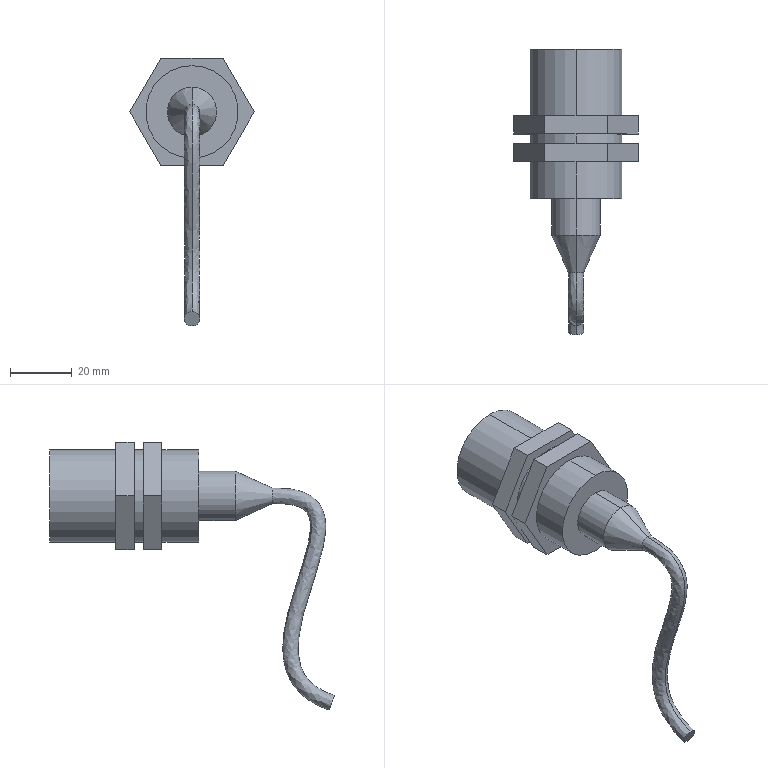Part | SolidWorks | features Boss 2, Extrusion 1, LPattern 1, Revolution 1, Sweep 1 | 1 solid | 31 faces | box 40.415 x 92.567 x 87.046 mm | volume 43733 mm3 | plane 19 | cylinder 8 | spline 2 | cone 2 | commonest cylinder face diameters 30 x6 16 x2
STEP:
#1=CARTESIAN_POINT('',(0.,-24.,-2.5));
#2=VERTEX_POINT('',#1);
#3=CARTESIAN_POINT('',(0.,-24.,2.5));
#4=VERTEX_POINT('',#3);
#5=CARTESIAN_POINT('',(0.,-24.,0.));
#6=DIRECTION('',(0.,-1.,0.));
#7=DIRECTION('',(0.,0.,-1.));
#8=AXIS2_PLACEMENT_3D('',#5,#6,#7);
#9=CIRCLE('',#8,2.5);
#10=EDGE_CURVE('',#2,#4,#9,.T.);
#11=ORIENTED_EDGE('',*,*,#10,.T.);
#12=CARTESIAN_POINT('',(0.,-44.067,-64.875));
#13=VERTEX_POINT('',#12);
#14=CARTESIAN_POINT('',(0.,-24.,2.5));
#15=CARTESIAN_POINT('',(0.,-26.65,2.597));
#16=CARTESIAN_POINT('',(0.,-28.95,2.46));
#17=CARTESIAN_POINT('',(0.,-32.981,1.702));
#18=CARTESIAN_POINT('',(0.,-34.722,1.075));
#19=CARTESIAN_POINT('',(0.,-37.648,-0.7421));
#20=CARTESIAN_POINT('',(0.,-38.817,-1.945));
#21=CARTESIAN_POINT('',(0.,-40.436,-4.701));
#22=CARTESIAN_POINT('',(0.,-40.89,-6.227));
#23=CARTESIAN_POINT('',(0.,-41.503,-10.943));
#24=CARTESIAN_POINT('',(0.,-40.983,-14.307));
#25=CARTESIAN_POINT('',(0.,-39.247,-21.447));
#26=CARTESIAN_POINT('',(0.,-37.999,-25.225));
#27=CARTESIAN_POINT('',(0.,-35.516,-32.906));
#28=CARTESIAN_POINT('',(0.,-34.279,-36.805));
#29=CARTESIAN_POINT('',(0.,-32.562,-44.284));
#30=CARTESIAN_POINT('',(0.,-32.091,-47.859));
#31=CARTESIAN_POINT('',(0.,-32.408,-52.584));
#32=CARTESIAN_POINT('',(0.,-32.68,-54.051));
#33=CARTESIAN_POINT('',(0.,-33.603,-56.751));
#34=CARTESIAN_POINT('',(0.,-34.251,-57.986));
#35=CARTESIAN_POINT('',(0.,-36.023,-60.274));
#36=CARTESIAN_POINT('',(0.,-37.151,-61.332));
#37=CARTESIAN_POINT('',(0.,-40.071,-63.265));
#38=CARTESIAN_POINT('',(0.,-41.867,-64.138));
#39=CARTESIAN_POINT('',(0.,-44.067,-64.875));
#40=B_SPLINE_CURVE_WITH_KNOTS('',3,(#14,#15,#16,#17,#18,#19,#20,#21,#22,#23,#24,#25,#26,#27,#28,#29,#30,#31,#32,#33,#34,#35,#36,#37,#38,#39),.UNSPECIFIED.,.F.,.F.,(4,2,2,2,2,2,2,2,2,2,2,2,4),(0.,0.0625,0.125,0.1875,0.25,0.375,0.5,0.625,0.75,0.8125,0.875,0.9375,1.),.UNSPECIFIED.);
#41=EDGE_CURVE('',#4,#13,#40,.T.);
#42=ORIENTED_EDGE('',*,*,#41,.T.);
#43=CARTESIAN_POINT('',(0.,-42.283,-69.546));
#44=VERTEX_POINT('',#43);
#45=CARTESIAN_POINT('',(0.,-43.175,-67.21));
#46=DIRECTION('',(0.,-0.9342,-0.3567));
#47=DIRECTION('',(0.,0.3567,-0.9342));
#48=AXIS2_PLACEMENT_3D('',#45,#46,#47);
#49=CIRCLE('',#48,2.5);
#50=EDGE_CURVE('',#44,#13,#49,.T.);
#51=ORIENTED_EDGE('',*,*,#50,.F.);
#52=CARTESIAN_POINT('',(0.,-24.,-2.5));
#53=CARTESIAN_POINT('',(0.,-26.373,-2.403));
#54=CARTESIAN_POINT('',(0.,-28.321,-2.523));
#55=CARTESIAN_POINT('',(0.,-31.428,-3.074));
#56=CARTESIAN_POINT('',(0.,-32.577,-3.503));
#57=CARTESIAN_POINT('',(0.,-34.264,-4.497));
#58=CARTESIAN_POINT('',(0.,-34.818,-5.05));
#59=CARTESIAN_POINT('',(0.,-35.671,-6.411));
#60=CARTESIAN_POINT('',(0.,-35.966,-7.244));
#61=CARTESIAN_POINT('',(0.,-36.423,-10.365));
#62=CARTESIAN_POINT('',(0.,-36.089,-13.236));
#63=CARTESIAN_POINT('',(0.,-34.517,-19.799));
#64=CARTESIAN_POINT('',(0.,-33.31,-23.491));
#65=CARTESIAN_POINT('',(0.,-30.816,-31.199));
#66=CARTESIAN_POINT('',(0.,-29.529,-35.22));
#67=CARTESIAN_POINT('',(0.,-27.663,-43.245));
#68=CARTESIAN_POINT('',(0.,-27.075,-47.254));
#69=CARTESIAN_POINT('',(0.,-27.418,-53.066));
#70=CARTESIAN_POINT('',(0.,-27.74,-54.971));
#71=CARTESIAN_POINT('',(0.,-28.945,-58.636));
#72=CARTESIAN_POINT('',(0.,-29.832,-60.395));
#73=CARTESIAN_POINT('',(0.,-32.262,-63.619));
#74=CARTESIAN_POINT('',(0.,-33.802,-65.079));
#75=CARTESIAN_POINT('',(0.,-37.539,-67.606));
#76=CARTESIAN_POINT('',(0.,-39.735,-68.676));
#77=CARTESIAN_POINT('',(0.,-42.283,-69.546));
#78=B_SPLINE_CURVE_WITH_KNOTS('',3,(#52,#53,#54,#55,#56,#57,#58,#59,#60,#61,#62,#63,#64,#65,#66,#67,#68,#69,#70,#71,#72,#73,#74,#75,#76,#77),.UNSPECIFIED.,.F.,.F.,(4,2,2,2,2,2,2,2,2,2,2,2,4),(0.,0.0625,0.125,0.1875,0.25,0.375,0.5,0.625,0.75,0.8125,0.875,0.9375,1.),.UNSPECIFIED.);
#79=EDGE_CURVE('',#2,#44,#78,.T.);
#80=ORIENTED_EDGE('',*,*,#79,.F.);
#81=EDGE_LOOP('',(#11,#42,#51,#80));
#82=FACE_OUTER_BOUND('',#81,.T.);
#83=CARTESIAN_POINT('',(0.,-24.,-2.5));
#84=CARTESIAN_POINT('',(0.,-26.373,-2.403));
#85=CARTESIAN_POINT('',(0.,-28.321,-2.523));
#86=CARTESIAN_POINT('',(0.,-31.428,-3.074));
#87=CARTESIAN_POINT('',(0.,-32.577,-3.503));
#88=CARTESIAN_POINT('',(0.,-34.264,-4.497));
#89=CARTESIAN_POINT('',(0.,-34.818,-5.05));
#90=CARTESIAN_POINT('',(0.,-35.671,-6.411));
#91=CARTESIAN_POINT('',(0.,-35.966,-7.244));
#92=CARTESIAN_POINT('',(0.,-36.423,-10.365));
#93=CARTESIAN_POINT('',(0.,-36.089,-13.236));
#94=CARTESIAN_POINT('',(0.,-34.517,-19.799));
#95=CARTESIAN_POINT('',(0.,-33.31,-23.491));
#96=CARTESIAN_POINT('',(0.,-30.816,-31.199));
#97=CARTESIAN_POINT('',(0.,-29.529,-35.22));
#98=CARTESIAN_POINT('',(0.,-27.663,-43.245));
#99=CARTESIAN_POINT('',(0.,-27.075,-47.254));
#100=CARTESIAN_POINT('',(0.,-27.418,-53.066));
#101=CARTESIAN_POINT('',(0.,-27.74,-54.971));
#102=CARTESIAN_POINT('',(0.,-28.945,-58.636));
#103=CARTESIAN_POINT('',(0.,-29.832,-60.395));
#104=CARTESIAN_POINT('',(0.,-32.262,-63.619));
#105=CARTESIAN_POINT('',(0.,-33.802,-65.079));
#106=CARTESIAN_POINT('',(0.,-37.539,-67.606));
#107=CARTESIAN_POINT('',(0.,-39.735,-68.676));
#108=CARTESIAN_POINT('',(0.,-42.283,-69.546));
#109=CARTESIAN_POINT('',(5.,-24.,-2.5));
#110=CARTESIAN_POINT('',(5.,-26.373,-2.403));
#111=CARTESIAN_POINT('',(5.,-28.321,-2.523));
#112=CARTESIAN_POINT('',(5.,-31.428,-3.074));
#113=CARTESIAN_POINT('',(5.,-32.577,-3.503));
#114=CARTESIAN_POINT('',(5.,-34.264,-4.497));
#115=CARTESIAN_POINT('',(5.,-34.818,-5.05));
#116=CARTESIAN_POINT('',(5.,-35.671,-6.411));
#117=CARTESIAN_POINT('',(5.,-35.966,-7.244));
#118=CARTESIAN_POINT('',(5.,-36.423,-10.365));
#119=CARTESIAN_POINT('',(5.,-36.089,-13.236));
#120=CARTESIAN_POINT('',(5.,-34.517,-19.799));
#121=CARTESIAN_POINT('',(5.,-33.31,-23.491));
#122=CARTESIAN_POINT('',(5.,-30.816,-31.199));
#123=CARTESIAN_POINT('',(5.,-29.529,-35.22));
#124=CARTESIAN_POINT('',(5.,-27.663,-43.245));
#125=CARTESIAN_POINT('',(5.,-27.075,-47.254));
#126=CARTESIAN_POINT('',(5.,-27.418,-53.066));
#127=CARTESIAN_POINT('',(5.,-27.74,-54.971));
#128=CARTESIAN_POINT('',(5.,-28.945,-58.636));
#129=CARTESIAN_POINT('',(5.,-29.832,-60.395));
#130=CARTESIAN_POINT('',(5.,-32.262,-63.619));
#131=CARTESIAN_POINT('',(5.,-33.802,-65.079));
#132=CARTESIAN_POINT('',(5.,-37.539,-67.606));
#133=CARTESIAN_POINT('',(5.,-39.735,-68.676));
#134=CARTESIAN_POINT('',(5.,-42.283,-69.546));
#135=CARTESIAN_POINT('',(5.,-24.,2.5));
#136=CARTESIAN_POINT('',(5.,-26.65,2.597));
#137=CARTESIAN_POINT('',(5.,-28.95,2.46));
#138=CARTESIAN_POINT('',(5.,-32.981,1.702));
#139=CARTESIAN_POINT('',(5.,-34.722,1.075));
#140=CARTESIAN_POINT('',(5.,-37.648,-0.7421));
#141=CARTESIAN_POINT('',(5.,-38.817,-1.945));
#142=CARTESIAN_POINT('',(5.,-40.436,-4.701));
#143=CARTESIAN_POINT('',(5.,-40.89,-6.227));
#144=CARTESIAN_POINT('',(5.,-41.503,-10.943));
#145=CARTESIAN_POINT('',(5.,-40.983,-14.307));
#146=CARTESIAN_POINT('',(5.,-39.247,-21.447));
#147=CARTESIAN_POINT('',(5.,-37.999,-25.225));
#148=CARTESIAN_POINT('',(5.,-35.516,-32.906));
#149=CARTESIAN_POINT('',(5.,-34.279,-36.805));
#150=CARTESIAN_POINT('',(5.,-32.562,-44.284));
#151=CARTESIAN_POINT('',(5.,-32.091,-47.859));
#152=CARTESIAN_POINT('',(5.,-32.408,-52.584));
#153=CARTESIAN_POINT('',(5.,-32.68,-54.051));
#154=CARTESIAN_POINT('',(5.,-33.603,-56.751));
#155=CARTESIAN_POINT('',(5.,-34.251,-57.986));
#156=CARTESIAN_POINT('',(5.,-36.023,-60.274));
#157=CARTESIAN_POINT('',(5.,-37.151,-61.332));
#158=CARTESIAN_POINT('',(5.,-40.071,-63.265));
#159=CARTESIAN_POINT('',(5.,-41.867,-64.138));
#160=CARTESIAN_POINT('',(5.,-44.067,-64.875));
#161=CARTESIAN_POINT('',(0.,-24.,2.5));
#162=CARTESIAN_POINT('',(0.,-26.65,2.597));
#163=CARTESIAN_POINT('',(0.,-28.95,2.46));
#164=CARTESIAN_POINT('',(0.,-32.981,1.702));
#165=CARTESIAN_POINT('',(0.,-34.722,1.075));
#166=CARTESIAN_POINT('',(0.,-37.648,-0.7421));
#167=CARTESIAN_POINT('',(0.,-38.817,-1.945));
#168=CARTESIAN_POINT('',(0.,-40.436,-4.701));
#169=CARTESIAN_POINT('',(0.,-40.89,-6.227));
#170=CARTESIAN_POINT('',(0.,-41.503,-10.943));
#171=CARTESIAN_POINT('',(0.,-40.983,-14.307));
#172=CARTESIAN_POINT('',(0.,-39.247,-21.447));
#173=CARTESIAN_POINT('',(0.,-37.999,-25.225));
#174=CARTESIAN_POINT('',(0.,-35.516,-32.906));
#175=CARTESIAN_POINT('',(0.,-34.279,-36.805));
#176=CARTESIAN_POINT('',(0.,-32.562,-44.284));
#177=CARTESIAN_POINT('',(0.,-32.091,-47.859));
#178=CARTESIAN_POINT('',(0.,-32.408,-52.584));
#179=CARTESIAN_POINT('',(0.,-32.68,-54.051));
#180=CARTESIAN_POINT('',(0.,-33.603,-56.751));
#181=CARTESIAN_POINT('',(0.,-34.251,-57.986));
#182=CARTESIAN_POINT('',(0.,-36.023,-60.274));
#183=CARTESIAN_POINT('',(0.,-37.151,-61.332));
#184=CARTESIAN_POINT('',(0.,-40.071,-63.265));
#185=CARTESIAN_POINT('',(0.,-41.867,-64.138));
#186=CARTESIAN_POINT('',(0.,-44.067,-64.875));
#187=CARTESIAN_POINT('',(-5.,-24.,2.5));
#188=CARTESIAN_POINT('',(-5.,-26.65,2.597));
#189=CARTESIAN_POINT('',(-5.,-28.95,2.46));
#190=CARTESIAN_POINT('',(-5.,-32.981,1.702));
#191=CARTESIAN_POINT('',(-5.,-34.722,1.075));
#192=CARTESIAN_POINT('',(-5.,-37.648,-0.7421));
#193=CARTESIAN_POINT('',(-5.,-38.817,-1.945));
#194=CARTESIAN_POINT('',(-5.,-40.436,-4.701));
#195=CARTESIAN_POINT('',(-5.,-40.89,-6.227));
#196=CARTESIAN_POINT('',(-5.,-41.503,-10.943));
#197=CARTESIAN_POINT('',(-5.,-40.983,-14.307));
#198=CARTESIAN_POINT('',(-5.,-39.247,-21.447));
#199=CARTESIAN_POINT('',(-5.,-37.999,-25.225));
#200=CARTESIAN_POINT('',(-5.,-35.516,-32.906));
#201=CARTESIAN_POINT('',(-5.,-34.279,-36.805));
#202=CARTESIAN_POINT('',(-5.,-32.562,-44.284));
#203=CARTESIAN_POINT('',(-5.,-32.091,-47.859));
#204=CARTESIAN_POINT('',(-5.,-32.408,-52.584));
#205=CARTESIAN_POINT('',(-5.,-32.68,-54.051));
#206=CARTESIAN_POINT('',(-5.,-33.603,-56.751));
#207=CARTESIAN_POINT('',(-5.,-34.251,-57.986));
#208=CARTESIAN_POINT('',(-5.,-36.023,-60.274));
#209=CARTESIAN_POINT('',(-5.,-37.151,-61.332));
#210=CARTESIAN_POINT('',(-5.,-40.071,-63.265));
#211=CARTESIAN_POINT('',(-5.,-41.867,-64.138));
#212=CARTESIAN_POINT('',(-5.,-44.067,-64.875));
#213=CARTESIAN_POINT('',(-5.,-24.,-2.5));
#214=CARTESIAN_POINT('',(-5.,-26.373,-2.403));
#215=CARTESIAN_POINT('',(-5.,-28.321,-2.523));
#216=CARTESIAN_POINT('',(-5.,-31.428,-3.074));
#217=CARTESIAN_POINT('',(-5.,-32.577,-3.503));
#218=CARTESIAN_POINT('',(-5.,-34.264,-4.497));
#219=CARTESIAN_POINT('',(-5.,-34.818,-5.05));
#220=CARTESIAN_POINT('',(-5.,-35.671,-6.411));
#221=CARTESIAN_POINT('',(-5.,-35.966,-7.244));
#222=CARTESIAN_POINT('',(-5.,-36.423,-10.365));
#223=CARTESIAN_POINT('',(-5.,-36.089,-13.236));
#224=CARTESIAN_POINT('',(-5.,-34.517,-19.799));
#225=CARTESIAN_POINT('',(-5.,-33.31,-23.491));
#226=CARTESIAN_POINT('',(-5.,-30.816,-31.199));
#227=CARTESIAN_POINT('',(-5.,-29.529,-35.22));
#228=CARTESIAN_POINT('',(-5.,-27.663,-43.245));
#229=CARTESIAN_POINT('',(-5.,-27.075,-47.254));
#230=CARTESIAN_POINT('',(-5.,-27.418,-53.066));
#231=CARTESIAN_POINT('',(-5.,-27.74,-54.971));
#232=CARTESIAN_POINT('',(-5.,-28.945,-58.636));
#233=CARTESIAN_POINT('',(-5.,-29.832,-60.395));
#234=CARTESIAN_POINT('',(-5.,-32.262,-63.619));
#235=CARTESIAN_POINT('',(-5.,-33.802,-65.079));
#236=CARTESIAN_POINT('',(-5.,-37.539,-67.606));
#237=CARTESIAN_POINT('',(-5.,-39.735,-68.676));
#238=CARTESIAN_POINT('',(-5.,-42.283,-69.546));
#239=CARTESIAN_POINT('',(0.,-24.,-2.5));
#240=CARTESIAN_POINT('',(0.,-26.373,-2.403));
#241=CARTESIAN_POINT('',(0.,-28.321,-2.523));
#242=CARTESIAN_POINT('',(0.,-31.428,-3.074));
#243=CARTESIAN_POINT('',(0.,-32.577,-3.503));
#244=CARTESIAN_POINT('',(0.,-34.264,-4.497));
#245=CARTESIAN_POINT('',(0.,-34.818,-5.05));
#246=CARTESIAN_POINT('',(0.,-35.671,-6.411));
#247=CARTESIAN_POINT('',(0.,-35.966,-7.244));
#248=CARTESIAN_POINT('',(0.,-36.423,-10.365));
#249=CARTESIAN_POINT('',(0.,-36.089,-13.236));
#250=CARTESIAN_POINT('',(0.,-34.517,-19.799));
#251=CARTESIAN_POINT('',(0.,-33.31,-23.491));
#252=CARTESIAN_POINT('',(0.,-30.816,-31.199));
#253=CARTESIAN_POINT('',(0.,-29.529,-35.22));
#254=CARTESIAN_POINT('',(0.,-27.663,-43.245));
#255=CARTESIAN_POINT('',(0.,-27.075,-47.254));
#256=CARTESIAN_POINT('',(0.,-27.418,-53.066));
#257=CARTESIAN_POINT('',(0.,-27.74,-54.971));
#258=CARTESIAN_POINT('',(0.,-28.945,-58.636));
#259=CARTESIAN_POINT('',(0.,-29.832,-60.395));
#260=CARTESIAN_POINT('',(0.,-32.262,-63.619));
#261=CARTESIAN_POINT('',(0.,-33.802,-65.079));
#262=CARTESIAN_POINT('',(0.,-37.539,-67.606));
#263=CARTESIAN_POINT('',(0.,-39.735,-68.676));
#264=CARTESIAN_POINT('',(0.,-42.283,-69.546));
#265=(BOUNDED_SURFACE()B_SPLINE_SURFACE(3,3,((#83,#84,#85,#86,#87,#88,#89,#90,#91,#92,#93,#94,#95,#96,#97,#98,#99,#100,#101,#102,#103,#104,#105,#106,#107,#108),(#109,#110,#111,#112,#113,#114,#115,#116,#117,#118,#119,#120,#121,#122,#123,#124,#125,#126,#127,#128,#129,#130,#131,#132,#133,#134),(#135,#136,#137,#138,#139,#140,#141,#142,#143,#144,#145,#146,#147,#148,#149,#150,#151,#152,#153,#154,#155,#156,#157,#158,#159,#160),(#161,#162,#163,#164,#165,#166,#167,#168,#169,#170,#171,#172,#173,#174,#175,#176,#177,#178,#179,#180,#181,#182,#183,#184,#185,#186),(#187,#188,#189,#190,#191,#192,#193,#194,#195,#196,#197,#198,#199,#200,#201,#202,#203,#204,#205,#206,#207,#208,#209,#210,#211,#212),(#213,#214,#215,#216,#217,#218,#219,#220,#221,#222,#223,#224,#225,#226,#227,#228,#229,#230,#231,#232,#233,#234,#235,#236,#237,#238),(#239,#240,#241,#242,#243,#244,#245,#246,#247,#248,#249,#250,#251,#252,#253,#254,#255,#256,#257,#258,#259,#260,#261,#262,#263,#264)),.UNSPECIFIED.,.T.,.F.,.F.)B_SPLINE_SURFACE_WITH_KNOTS((4,3,4),(4,2,2,2,2,2,2,2,2,2,2,2,4),(0.,0.5,1.),(0.,0.0625,0.125,0.1875,0.25,0.375,0.5,0.625,0.75,0.8125,0.875,0.9375,1.),.UNSPECIFIED.)GEOMETRIC_REPRESENTATION_ITEM()RATIONAL_B_SPLINE_SURFACE(((1.,1.,1.,1.,1.,1.,1.,1.,1.,1.,1.,1.,1.,1.,1.,1.,1.,1.,1.,1.,1.,1.,1.,1.,1.,1.),(0.3333,0.3333,0.3333,0.3333,0.3333,0.3333,0.3333,0.3333,0.3333,0.3333,0.3333,0.3333,0.3333,0.3333,0.3333,0.3333,0.3333,0.3333,0.3333,0.3333,0.3333,0.3333,0.3333,0.3333,0.3333,0.3333),(0.3333,0.3333,0.3333,0.3333,0.3333,0.3333,0.3333,0.3333,0.3333,0.3333,0.3333,0.3333,0.3333,0.3333,0.3333,0.3333,0.3333,0.3333,0.3333,0.3333,0.3333,0.3333,0.3333,0.3333,0.3333,0.3333),(1.,1.,1.,1.,1.,1.,1.,1.,1.,1.,1.,1.,1.,1.,1.,1.,1.,1.,1.,1.,1.,1.,1.,1.,1.,1.),(0.3333,0.3333,0.3333,0.3333,0.3333,0.3333,0.3333,0.3333,0.3333,0.3333,0.3333,0.3333,0.3333,0.3333,0.3333,0.3333,0.3333,0.3333,0.3333,0.3333,0.3333,0.3333,0.3333,0.3333,0.3333,0.3333),(0.3333,0.3333,0.3333,0.3333,0.3333,0.3333,0.3333,0.3333,0.3333,0.3333,0.3333,0.3333,0.3333,0.3333,0.3333,0.3333,0.3333,0.3333,0.3333,0.3333,0.3333,0.3333,0.3333,0.3333,0.3333,0.3333),(1.,1.,1.,1.,1.,1.,1.,1.,1.,1.,1.,1.,1.,1.,1.,1.,1.,1.,1.,1.,1.,1.,1.,1.,1.,1.)))REPRESENTATION_ITEM('')SURFACE());
#266=ADVANCED_FACE('',(#82),#265,.T.);
#267=ORIENTED_EDGE('',*,*,#10,.F.);
#268=CARTESIAN_POINT('',(0.,-11.832,-8.));
#269=VERTEX_POINT('',#268);
#270=CARTESIAN_POINT('',(0.,-24.,-2.5));
#271=DIRECTION('',(0.,0.9112,-0.4119));
#272=VECTOR('',#271,1000.);
#273=LINE('',#270,#272);
#274=EDGE_CURVE('',#2,#269,#273,.T.);
#275=ORIENTED_EDGE('',*,*,#274,.T.);
#276=CARTESIAN_POINT('',(0.,-11.832,8.));
#277=VERTEX_POINT('',#276);
#278=CARTESIAN_POINT('',(0.,-11.832,0.));
#279=DIRECTION('',(0.,1.,0.));
#280=DIRECTION('',(0.,0.,1.));
#281=AXIS2_PLACEMENT_3D('',#278,#279,#280);
#282=CIRCLE('',#281,8.);
#283=EDGE_CURVE('',#277,#269,#282,.T.);
#284=ORIENTED_EDGE('',*,*,#283,.F.);
#285=CARTESIAN_POINT('',(0.,-24.,2.5));
#286=DIRECTION('',(0.,0.9112,0.4119));
#287=VECTOR('',#286,1000.);
#288=LINE('',#285,#287);
#289=EDGE_CURVE('',#4,#277,#288,.T.);
#290=ORIENTED_EDGE('',*,*,#289,.F.);
#291=EDGE_LOOP('',(#267,#275,#284,#290));
#292=FACE_OUTER_BOUND('',#291,.T.);
#293=CARTESIAN_POINT('',(0.,-24.,0.));
#294=DIRECTION('',(0.,1.,0.));
#295=DIRECTION('',(0.,0.,1.));
#296=AXIS2_PLACEMENT_3D('',#293,#294,#295);
#297=CONICAL_SURFACE('',#296,2.5,0.4245);
#298=ADVANCED_FACE('',(#292),#297,.T.);
#299=ORIENTED_EDGE('',*,*,#283,.T.);
#300=CARTESIAN_POINT('',(0.,0.,-8.));
#301=VERTEX_POINT('',#300);
#302=CARTESIAN_POINT('',(0.,0.,-8.));
#303=DIRECTION('',(0.,1.,0.));
#304=VECTOR('',#303,1000.);
#305=LINE('',#302,#304);
#306=EDGE_CURVE('',#269,#301,#305,.T.);
#307=ORIENTED_EDGE('',*,*,#306,.T.);
#308=CARTESIAN_POINT('',(0.,0.,8.));
#309=VERTEX_POINT('',#308);
#310=CARTESIAN_POINT('',(0.,0.,0.));
#311=DIRECTION('',(0.,-1.,0.));
#312=DIRECTION('',(0.,0.,1.));
#313=AXIS2_PLACEMENT_3D('',#310,#311,#312);
#314=CIRCLE('',#313,8.);
#315=EDGE_CURVE('',#301,#309,#314,.T.);
#316=ORIENTED_EDGE('',*,*,#315,.T.);
#317=CARTESIAN_POINT('',(0.,0.,8.));
#318=DIRECTION('',(0.,1.,0.));
#319=VECTOR('',#318,1000.);
#320=LINE('',#317,#319);
#321=EDGE_CURVE('',#277,#309,#320,.T.);
#322=ORIENTED_EDGE('',*,*,#321,.F.);
#323=EDGE_LOOP('',(#299,#307,#316,#322));
#324=FACE_OUTER_BOUND('',#323,.T.);
#325=CARTESIAN_POINT('',(0.,0.,0.));
#326=DIRECTION('',(0.,1.,0.));
#327=DIRECTION('',(0.,0.,1.));
#328=AXIS2_PLACEMENT_3D('',#325,#326,#327);
#329=CYLINDRICAL_SURFACE('',#328,8.);
#330=ADVANCED_FACE('',(#324),#329,.T.);
#331=CARTESIAN_POINT('',(0.,48.5,15.));
#332=VERTEX_POINT('',#331);
#333=CARTESIAN_POINT('',(0.,48.5,-15.));
#334=VERTEX_POINT('',#333);
#335=CARTESIAN_POINT('',(0.,48.5,0.));
#336=DIRECTION('',(0.,1.,0.));
#337=DIRECTION('',(0.,0.,1.));
#338=AXIS2_PLACEMENT_3D('',#335,#336,#337);
#339=CIRCLE('',#338,15.);
#340=EDGE_CURVE('',#332,#334,#339,.T.);
#341=ORIENTED_EDGE('',*,*,#340,.F.);
#342=CARTESIAN_POINT('',(0.,27.,15.));
#343=VERTEX_POINT('',#342);
#344=CARTESIAN_POINT('',(0.,48.5,15.));
#345=DIRECTION('',(0.,-1.,0.));
#346=VECTOR('',#345,1000.);
#347=LINE('',#344,#346);
#348=EDGE_CURVE('',#332,#343,#347,.T.);
#349=ORIENTED_EDGE('',*,*,#348,.T.);
#350=CARTESIAN_POINT('',(0.,27.,-15.));
#351=VERTEX_POINT('',#350);
#352=CARTESIAN_POINT('',(0.,27.,0.));
#353=DIRECTION('',(0.,1.,0.));
#354=DIRECTION('',(0.,0.,1.));
#355=AXIS2_PLACEMENT_3D('',#352,#353,#354);
#356=CIRCLE('',#355,15.);
#357=EDGE_CURVE('',#343,#351,#356,.T.);
#358=ORIENTED_EDGE('',*,*,#357,.T.);
#359=CARTESIAN_POINT('',(0.,48.5,-15.));
#360=DIRECTION('',(0.,-1.,0.));
#361=VECTOR('',#360,1000.);
#362=LINE('',#359,#361);
#363=EDGE_CURVE('',#334,#351,#362,.T.);
#364=ORIENTED_EDGE('',*,*,#363,.F.);
#365=EDGE_LOOP('',(#341,#349,#358,#364));
#366=FACE_OUTER_BOUND('',#365,.T.);
#367=CARTESIAN_POINT('',(0.,48.5,0.));
#368=DIRECTION('',(0.,-1.,0.));
#369=DIRECTION('',(0.,0.,-1.));
#370=AXIS2_PLACEMENT_3D('',#367,#368,#369);
#371=CYLINDRICAL_SURFACE('',#370,15.);
#372=ADVANCED_FACE('',(#366),#371,.T.);
#373=CARTESIAN_POINT('',(0.,12.,15.));
#374=VERTEX_POINT('',#373);
#375=CARTESIAN_POINT('',(0.,12.,-15.));
#376=VERTEX_POINT('',#375);
#377=CARTESIAN_POINT('',(0.,12.,0.));
#378=DIRECTION('',(0.,1.,0.));
#379=DIRECTION('',(0.,0.,1.));
#380=AXIS2_PLACEMENT_3D('',#377,#378,#379);
#381=CIRCLE('',#380,15.);
#382=EDGE_CURVE('',#374,#376,#381,.T.);
#383=ORIENTED_EDGE('',*,*,#382,.F.);
#384=CARTESIAN_POINT('',(0.,0.,15.));
#385=VERTEX_POINT('',#384);
#386=CARTESIAN_POINT('',(0.,48.5,15.));
#387=DIRECTION('',(0.,-1.,0.));
#388=VECTOR('',#387,1000.);
#389=LINE('',#386,#388);
#390=EDGE_CURVE('',#374,#385,#389,.T.);
#391=ORIENTED_EDGE('',*,*,#390,.T.);
#392=CARTESIAN_POINT('',(0.,0.,-15.));
#393=VERTEX_POINT('',#392);
#394=CARTESIAN_POINT('',(0.,0.,0.));
#395=DIRECTION('',(0.,1.,0.));
#396=DIRECTION('',(0.,0.,1.));
#397=AXIS2_PLACEMENT_3D('',#394,#395,#396);
#398=CIRCLE('',#397,15.);
#399=EDGE_CURVE('',#385,#393,#398,.T.);
#400=ORIENTED_EDGE('',*,*,#399,.T.);
#401=CARTESIAN_POINT('',(0.,48.5,-15.));
#402=DIRECTION('',(0.,-1.,0.));
#403=VECTOR('',#402,1000.);
#404=LINE('',#401,#403);
#405=EDGE_CURVE('',#376,#393,#404,.T.);
#406=ORIENTED_EDGE('',*,*,#405,.F.);
#407=EDGE_LOOP('',(#383,#391,#400,#406));
#408=FACE_OUTER_BOUND('',#407,.T.);
#409=CARTESIAN_POINT('',(0.,48.5,0.));
#410=DIRECTION('',(0.,-1.,0.));
#411=DIRECTION('',(0.,0.,-1.));
#412=AXIS2_PLACEMENT_3D('',#409,#410,#411);
#413=CYLINDRICAL_SURFACE('',#412,15.);
#414=ADVANCED_FACE('',(#408),#413,.T.);
#415=CARTESIAN_POINT('',(0.,21.,15.));
#416=VERTEX_POINT('',#415);
#417=CARTESIAN_POINT('',(0.,21.,-15.));
#418=VERTEX_POINT('',#417);
#419=CARTESIAN_POINT('',(0.,21.,0.));
#420=DIRECTION('',(0.,1.,0.));
#421=DIRECTION('',(0.,0.,1.));
#422=AXIS2_PLACEMENT_3D('',#419,#420,#421);
#423=CIRCLE('',#422,15.);
#424=EDGE_CURVE('',#416,#418,#423,.T.);
#425=ORIENTED_EDGE('',*,*,#424,.F.);
#426=CARTESIAN_POINT('',(0.,18.,15.));
#427=VERTEX_POINT('',#426);
#428=CARTESIAN_POINT('',(0.,48.5,15.));
#429=DIRECTION('',(0.,-1.,0.));
#430=VECTOR('',#429,1000.);
#431=LINE('',#428,#430);
#432=EDGE_CURVE('',#416,#427,#431,.T.);
#433=ORIENTED_EDGE('',*,*,#432,.T.);
#434=CARTESIAN_POINT('',(0.,18.,-15.));
#435=VERTEX_POINT('',#434);
#436=CARTESIAN_POINT('',(0.,18.,0.));
#437=DIRECTION('',(0.,1.,0.));
#438=DIRECTION('',(0.,0.,1.));
#439=AXIS2_PLACEMENT_3D('',#436,#437,#438);
#440=CIRCLE('',#439,15.);
#441=EDGE_CURVE('',#427,#435,#440,.T.);
#442=ORIENTED_EDGE('',*,*,#441,.T.);
#443=CARTESIAN_POINT('',(0.,48.5,-15.));
#444=DIRECTION('',(0.,-1.,0.));
#445=VECTOR('',#444,1000.);
#446=LINE('',#443,#445);
#447=EDGE_CURVE('',#418,#435,#446,.T.);
#448=ORIENTED_EDGE('',*,*,#447,.F.);
#449=EDGE_LOOP('',(#425,#433,#442,#448));
#450=FACE_OUTER_BOUND('',#449,.T.);
#451=CARTESIAN_POINT('',(0.,48.5,0.));
#452=DIRECTION('',(0.,-1.,0.));
#453=DIRECTION('',(0.,0.,-1.));
#454=AXIS2_PLACEMENT_3D('',#451,#452,#453);
#455=CYLINDRICAL_SURFACE('',#454,15.);
#456=ADVANCED_FACE('',(#450),#455,.T.);
#457=CARTESIAN_POINT('',(0.,0.,0.));
#458=DIRECTION('',(0.,1.,0.));
#459=DIRECTION('',(0.,0.,1.));
#460=AXIS2_PLACEMENT_3D('',#457,#458,#459);
#461=CIRCLE('',#460,15.);
#462=EDGE_CURVE('',#393,#385,#461,.T.);
#463=ORIENTED_EDGE('',*,*,#462,.F.);
#464=ORIENTED_EDGE('',*,*,#399,.F.);
#465=EDGE_LOOP('',(#463,#464));
#466=FACE_OUTER_BOUND('',#465,.T.);
#467=CARTESIAN_POINT('',(0.,0.,0.));
#468=DIRECTION('',(0.,-1.,0.));
#469=DIRECTION('',(0.,0.,1.));
#470=AXIS2_PLACEMENT_3D('',#467,#468,#469);
#471=CIRCLE('',#470,8.);
#472=EDGE_CURVE('',#309,#301,#471,.T.);
#473=ORIENTED_EDGE('',*,*,#472,.F.);
#474=ORIENTED_EDGE('',*,*,#315,.F.);
#475=EDGE_LOOP('',(#473,#474));
#476=FACE_BOUND('',#475,.T.);
#477=CARTESIAN_POINT('',(0.,0.,0.));
#478=DIRECTION('',(0.,1.,0.));
#479=DIRECTION('',(0.,0.,1.));
#480=AXIS2_PLACEMENT_3D('',#477,#478,#479);
#481=PLANE('',#480);
#482=ADVANCED_FACE('',(#466,#476),#481,.F.);
#483=ORIENTED_EDGE('',*,*,#432,.F.);
#484=CARTESIAN_POINT('',(0.,21.,0.));
#485=DIRECTION('',(0.,1.,0.));
#486=DIRECTION('',(0.,0.,1.));
#487=AXIS2_PLACEMENT_3D('',#484,#485,#486);
#488=CIRCLE('',#487,15.);
#489=EDGE_CURVE('',#418,#416,#488,.T.);
#490=ORIENTED_EDGE('',*,*,#489,.F.);
#491=ORIENTED_EDGE('',*,*,#447,.T.);
#492=CARTESIAN_POINT('',(0.,18.,0.));
#493=DIRECTION('',(0.,1.,0.));
#494=DIRECTION('',(0.,0.,1.));
#495=AXIS2_PLACEMENT_3D('',#492,#493,#494);
#496=CIRCLE('',#495,15.);
#497=EDGE_CURVE('',#435,#427,#496,.T.);
#498=ORIENTED_EDGE('',*,*,#497,.T.);
#499=EDGE_LOOP('',(#483,#490,#491,#498));
#500=FACE_OUTER_BOUND('',#499,.T.);
#501=CARTESIAN_POINT('',(0.,48.5,0.));
#502=DIRECTION('',(0.,-1.,0.));
#503=DIRECTION('',(0.,0.,-1.));
#504=AXIS2_PLACEMENT_3D('',#501,#502,#503);
#505=CYLINDRICAL_SURFACE('',#504,15.);
#506=ADVANCED_FACE('',(#500),#505,.T.);
#507=CARTESIAN_POINT('',(-10.104,18.,17.5));
#508=VERTEX_POINT('',#507);
#509=CARTESIAN_POINT('',(10.104,18.,17.5));
#510=VERTEX_POINT('',#509);
#511=CARTESIAN_POINT('',(-10.104,18.,17.5));
#512=DIRECTION('',(1.,0.,0.));
#513=VECTOR('',#512,1000.);
#514=LINE('',#511,#513);
#515=EDGE_CURVE('',#508,#510,#514,.T.);
#516=ORIENTED_EDGE('',*,*,#515,.T.);
#517=CARTESIAN_POINT('',(20.207,18.,0.));
#518=VERTEX_POINT('',#517);
#519=CARTESIAN_POINT('',(10.104,18.,17.5));
#520=DIRECTION('',(0.5,0.,-0.866));
#521=VECTOR('',#520,1000.);
#522=LINE('',#519,#521);
#523=EDGE_CURVE('',#510,#518,#522,.T.);
#524=ORIENTED_EDGE('',*,*,#523,.T.);
#525=CARTESIAN_POINT('',(10.104,18.,-17.5));
#526=VERTEX_POINT('',#525);
#527=CARTESIAN_POINT('',(20.207,18.,0.));
#528=DIRECTION('',(-0.5,0.,-0.866));
#529=VECTOR('',#528,1000.);
#530=LINE('',#527,#529);
#531=EDGE_CURVE('',#518,#526,#530,.T.);
#532=ORIENTED_EDGE('',*,*,#531,.T.);
#533=CARTESIAN_POINT('',(-10.104,18.,-17.5));
#534=VERTEX_POINT('',#533);
#535=CARTESIAN_POINT('',(10.104,18.,-17.5));
#536=DIRECTION('',(-1.,0.,0.));
#537=VECTOR('',#536,1000.);
#538=LINE('',#535,#537);
#539=EDGE_CURVE('',#526,#534,#538,.T.);
#540=ORIENTED_EDGE('',*,*,#539,.T.);
#541=CARTESIAN_POINT('',(-20.207,18.,0.));
#542=VERTEX_POINT('',#541);
#543=CARTESIAN_POINT('',(-10.104,18.,-17.5));
#544=DIRECTION('',(-0.5,0.,0.866));
#545=VECTOR('',#544,1000.);
#546=LINE('',#543,#545);
#547=EDGE_CURVE('',#534,#542,#546,.T.);
#548=ORIENTED_EDGE('',*,*,#547,.T.);
#549=CARTESIAN_POINT('',(-20.207,18.,0.));
#550=DIRECTION('',(0.5,0.,0.866));
#551=VECTOR('',#550,1000.);
#552=LINE('',#549,#551);
#553=EDGE_CURVE('',#542,#508,#552,.T.);
#554=ORIENTED_EDGE('',*,*,#553,.T.);
#555=EDGE_LOOP('',(#516,#524,#532,#540,#548,#554));
#556=FACE_OUTER_BOUND('',#555,.T.);
#557=ORIENTED_EDGE('',*,*,#497,.F.);
#558=ORIENTED_EDGE('',*,*,#441,.F.);
#559=EDGE_LOOP('',(#557,#558));
#560=FACE_BOUND('',#559,.T.);
#561=CARTESIAN_POINT('',(10.104,18.,17.5));
#562=DIRECTION('',(0.,1.,0.));
#563=DIRECTION('',(0.,0.,1.));
#564=AXIS2_PLACEMENT_3D('',#561,#562,#563);
#565=PLANE('',#564);
#566=ADVANCED_FACE('',(#556,#560),#565,.T.);
#567=CARTESIAN_POINT('',(-10.104,12.,17.5));
#568=VERTEX_POINT('',#567);
#569=CARTESIAN_POINT('',(10.104,12.,17.5));
#570=VERTEX_POINT('',#569);
#571=CARTESIAN_POINT('',(-10.104,12.,17.5));
#572=DIRECTION('',(1.,0.,0.));
#573=VECTOR('',#572,1000.);
#574=LINE('',#571,#573);
#575=EDGE_CURVE('',#568,#570,#574,.T.);
#576=ORIENTED_EDGE('',*,*,#575,.F.);
#577=CARTESIAN_POINT('',(-20.207,12.,0.));
#578=VERTEX_POINT('',#577);
#579=CARTESIAN_POINT('',(-20.207,12.,0.));
#580=DIRECTION('',(0.5,0.,0.866));
#581=VECTOR('',#580,1000.);
#582=LINE('',#579,#581);
#583=EDGE_CURVE('',#578,#568,#582,.T.);
#584=ORIENTED_EDGE('',*,*,#583,.F.);
#585=CARTESIAN_POINT('',(-10.104,12.,-17.5));
#586=VERTEX_POINT('',#585);
#587=CARTESIAN_POINT('',(-10.104,12.,-17.5));
#588=DIRECTION('',(-0.5,0.,0.866));
#589=VECTOR('',#588,1000.);
#590=LINE('',#587,#589);
#591=EDGE_CURVE('',#586,#578,#590,.T.);
#592=ORIENTED_EDGE('',*,*,#591,.F.);
#593=CARTESIAN_POINT('',(10.104,12.,-17.5));
#594=VERTEX_POINT('',#593);
#595=CARTESIAN_POINT('',(10.104,12.,-17.5));
#596=DIRECTION('',(-1.,0.,0.));
#597=VECTOR('',#596,1000.);
#598=LINE('',#595,#597);
#599=EDGE_CURVE('',#594,#586,#598,.T.);
#600=ORIENTED_EDGE('',*,*,#599,.F.);
#601=CARTESIAN_POINT('',(20.207,12.,0.));
#602=VERTEX_POINT('',#601);
#603=CARTESIAN_POINT('',(20.207,12.,0.));
#604=DIRECTION('',(-0.5,0.,-0.866));
#605=VECTOR('',#604,1000.);
#606=LINE('',#603,#605);
#607=EDGE_CURVE('',#602,#594,#606,.T.);
#608=ORIENTED_EDGE('',*,*,#607,.F.);
#609=CARTESIAN_POINT('',(10.104,12.,17.5));
#610=DIRECTION('',(0.5,0.,-0.866));
#611=VECTOR('',#610,1000.);
#612=LINE('',#609,#611);
#613=EDGE_CURVE('',#570,#602,#612,.T.);
#614=ORIENTED_EDGE('',*,*,#613,.F.);
#615=EDGE_LOOP('',(#576,#584,#592,#600,#608,#614));
#616=FACE_OUTER_BOUND('',#615,.T.);
#617=CARTESIAN_POINT('',(0.,12.,0.));
#618=DIRECTION('',(0.,1.,0.));
#619=DIRECTION('',(0.,0.,1.));
#620=AXIS2_PLACEMENT_3D('',#617,#618,#619);
#621=CIRCLE('',#620,15.);
#622=EDGE_CURVE('',#376,#374,#621,.T.);
#623=ORIENTED_EDGE('',*,*,#622,.T.);
#624=ORIENTED_EDGE('',*,*,#382,.T.);
#625=EDGE_LOOP('',(#623,#624));
#626=FACE_BOUND('',#625,.T.);
#627=CARTESIAN_POINT('',(10.104,12.,17.5));
#628=DIRECTION('',(0.,1.,0.));
#629=DIRECTION('',(0.,0.,1.));
#630=AXIS2_PLACEMENT_3D('',#627,#628,#629);
#631=PLANE('',#630);
#632=ADVANCED_FACE('',(#616,#626),#631,.F.);
#633=ORIENTED_EDGE('',*,*,#575,.T.);
#634=CARTESIAN_POINT('',(10.104,18.,17.5));
#635=DIRECTION('',(0.,-1.,0.));
#636=VECTOR('',#635,1000.);
#637=LINE('',#634,#636);
#638=EDGE_CURVE('',#510,#570,#637,.T.);
#639=ORIENTED_EDGE('',*,*,#638,.F.);
#640=ORIENTED_EDGE('',*,*,#515,.F.);
#641=CARTESIAN_POINT('',(-10.104,18.,17.5));
#642=DIRECTION('',(0.,-1.,0.));
#643=VECTOR('',#642,1000.);
#644=LINE('',#641,#643);
#645=EDGE_CURVE('',#508,#568,#644,.T.);
#646=ORIENTED_EDGE('',*,*,#645,.T.);
#647=EDGE_LOOP('',(#633,#639,#640,#646));
#648=FACE_OUTER_BOUND('',#647,.T.);
#649=CARTESIAN_POINT('',(-10.104,18.,17.5));
#650=DIRECTION('',(0.,0.,-1.));
#651=DIRECTION('',(-1.,0.,0.));
#652=AXIS2_PLACEMENT_3D('',#649,#650,#651);
#653=PLANE('',#652);
#654=ADVANCED_FACE('',(#648),#653,.F.);
#655=ORIENTED_EDGE('',*,*,#613,.T.);
#656=CARTESIAN_POINT('',(20.207,18.,0.));
#657=DIRECTION('',(0.,-1.,0.));
#658=VECTOR('',#657,1000.);
#659=LINE('',#656,#658);
#660=EDGE_CURVE('',#518,#602,#659,.T.);
#661=ORIENTED_EDGE('',*,*,#660,.F.);
#662=ORIENTED_EDGE('',*,*,#523,.F.);
#663=ORIENTED_EDGE('',*,*,#638,.T.);
#664=EDGE_LOOP('',(#655,#661,#662,#663));
#665=FACE_OUTER_BOUND('',#664,.T.);
#666=CARTESIAN_POINT('',(10.104,18.,17.5));
#667=DIRECTION('',(-0.866,0.,-0.5));
#668=DIRECTION('',(-0.5,0.,0.866));
#669=AXIS2_PLACEMENT_3D('',#666,#667,#668);
#670=PLANE('',#669);
#671=ADVANCED_FACE('',(#665),#670,.F.);
#672=ORIENTED_EDGE('',*,*,#607,.T.);
#673=CARTESIAN_POINT('',(10.104,18.,-17.5));
#674=DIRECTION('',(0.,-1.,0.));
#675=VECTOR('',#674,1000.);
#676=LINE('',#673,#675);
#677=EDGE_CURVE('',#526,#594,#676,.T.);
#678=ORIENTED_EDGE('',*,*,#677,.F.);
#679=ORIENTED_EDGE('',*,*,#531,.F.);
#680=ORIENTED_EDGE('',*,*,#660,.T.);
#681=EDGE_LOOP('',(#672,#678,#679,#680));
#682=FACE_OUTER_BOUND('',#681,.T.);
#683=CARTESIAN_POINT('',(20.207,18.,0.));
#684=DIRECTION('',(-0.866,0.,0.5));
#685=DIRECTION('',(0.5,0.,0.866));
#686=AXIS2_PLACEMENT_3D('',#683,#684,#685);
#687=PLANE('',#686);
#688=ADVANCED_FACE('',(#682),#687,.F.);
#689=ORIENTED_EDGE('',*,*,#599,.T.);
#690=CARTESIAN_POINT('',(-10.104,18.,-17.5));
#691=DIRECTION('',(0.,-1.,0.));
#692=VECTOR('',#691,1000.);
#693=LINE('',#690,#692);
#694=EDGE_CURVE('',#534,#586,#693,.T.);
#695=ORIENTED_EDGE('',*,*,#694,.F.);
#696=ORIENTED_EDGE('',*,*,#539,.F.);
#697=ORIENTED_EDGE('',*,*,#677,.T.);
#698=EDGE_LOOP('',(#689,#695,#696,#697));
#699=FACE_OUTER_BOUND('',#698,.T.);
#700=CARTESIAN_POINT('',(10.104,18.,-17.5));
#701=DIRECTION('',(0.,0.,1.));
#702=DIRECTION('',(1.,0.,0.));
#703=AXIS2_PLACEMENT_3D('',#700,#701,#702);
#704=PLANE('',#703);
#705=ADVANCED_FACE('',(#699),#704,.F.);
#706=ORIENTED_EDGE('',*,*,#591,.T.);
#707=CARTESIAN_POINT('',(-20.207,18.,0.));
#708=DIRECTION('',(0.,-1.,0.));
#709=VECTOR('',#708,1000.);
#710=LINE('',#707,#709);
#711=EDGE_CURVE('',#542,#578,#710,.T.);
#712=ORIENTED_EDGE('',*,*,#711,.F.);
#713=ORIENTED_EDGE('',*,*,#547,.F.);
#714=ORIENTED_EDGE('',*,*,#694,.T.);
#715=EDGE_LOOP('',(#706,#712,#713,#714));
#716=FACE_OUTER_BOUND('',#715,.T.);
#717=CARTESIAN_POINT('',(-10.104,18.,-17.5));
#718=DIRECTION('',(0.866,0.,0.5));
#719=DIRECTION('',(0.5,0.,-0.866));
#720=AXIS2_PLACEMENT_3D('',#717,#718,#719);
#721=PLANE('',#720);
#722=ADVANCED_FACE('',(#716),#721,.F.);
#723=ORIENTED_EDGE('',*,*,#583,.T.);
#724=ORIENTED_EDGE('',*,*,#645,.F.);
#725=ORIENTED_EDGE('',*,*,#553,.F.);
#726=ORIENTED_EDGE('',*,*,#711,.T.);
#727=EDGE_LOOP('',(#723,#724,#725,#726));
#728=FACE_OUTER_BOUND('',#727,.T.);
#729=CARTESIAN_POINT('',(-20.207,18.,0.));
#730=DIRECTION('',(0.866,0.,-0.5));
#731=DIRECTION('',(-0.5,0.,-0.866));
#732=AXIS2_PLACEMENT_3D('',#729,#730,#731);
#733=PLANE('',#732);
#734=ADVANCED_FACE('',(#728),#733,.F.);
#735=ORIENTED_EDGE('',*,*,#390,.F.);
#736=ORIENTED_EDGE('',*,*,#622,.F.);
#737=ORIENTED_EDGE('',*,*,#405,.T.);
#738=ORIENTED_EDGE('',*,*,#462,.T.);
#739=EDGE_LOOP('',(#735,#736,#737,#738));
#740=FACE_OUTER_BOUND('',#739,.T.);
#741=CARTESIAN_POINT('',(0.,48.5,0.));
#742=DIRECTION('',(0.,-1.,0.));
#743=DIRECTION('',(0.,0.,-1.));
#744=AXIS2_PLACEMENT_3D('',#741,#742,#743);
#745=CYLINDRICAL_SURFACE('',#744,15.);
#746=ADVANCED_FACE('',(#740),#745,.T.);
#747=CARTESIAN_POINT('',(-10.104,27.,17.5));
#748=VERTEX_POINT('',#747);
#749=CARTESIAN_POINT('',(10.104,27.,17.5));
#750=VERTEX_POINT('',#749);
#751=CARTESIAN_POINT('',(-10.104,27.,17.5));
#752=DIRECTION('',(1.,0.,0.));
#753=VECTOR('',#752,1000.);
#754=LINE('',#751,#753);
#755=EDGE_CURVE('',#748,#750,#754,.T.);
#756=ORIENTED_EDGE('',*,*,#755,.T.);
#757=CARTESIAN_POINT('',(20.207,27.,0.));
#758=VERTEX_POINT('',#757);
#759=CARTESIAN_POINT('',(10.104,27.,17.5));
#760=DIRECTION('',(0.5,0.,-0.866));
#761=VECTOR('',#760,1000.);
#762=LINE('',#759,#761);
#763=EDGE_CURVE('',#750,#758,#762,.T.);
#764=ORIENTED_EDGE('',*,*,#763,.T.);
#765=CARTESIAN_POINT('',(10.104,27.,-17.5));
#766=VERTEX_POINT('',#765);
#767=CARTESIAN_POINT('',(20.207,27.,0.));
#768=DIRECTION('',(-0.5,0.,-0.866));
#769=VECTOR('',#768,1000.);
#770=LINE('',#767,#769);
#771=EDGE_CURVE('',#758,#766,#770,.T.);
#772=ORIENTED_EDGE('',*,*,#771,.T.);
#773=CARTESIAN_POINT('',(-10.104,27.,-17.5));
#774=VERTEX_POINT('',#773);
#775=CARTESIAN_POINT('',(10.104,27.,-17.5));
#776=DIRECTION('',(-1.,0.,0.));
#777=VECTOR('',#776,1000.);
#778=LINE('',#775,#777);
#779=EDGE_CURVE('',#766,#774,#778,.T.);
#780=ORIENTED_EDGE('',*,*,#779,.T.);
#781=CARTESIAN_POINT('',(-20.207,27.,0.));
#782=VERTEX_POINT('',#781);
#783=CARTESIAN_POINT('',(-10.104,27.,-17.5));
#784=DIRECTION('',(-0.5,0.,0.866));
#785=VECTOR('',#784,1000.);
#786=LINE('',#783,#785);
#787=EDGE_CURVE('',#774,#782,#786,.T.);
#788=ORIENTED_EDGE('',*,*,#787,.T.);
#789=CARTESIAN_POINT('',(-20.207,27.,0.));
#790=DIRECTION('',(0.5,0.,0.866));
#791=VECTOR('',#790,1000.);
#792=LINE('',#789,#791);
#793=EDGE_CURVE('',#782,#748,#792,.T.);
#794=ORIENTED_EDGE('',*,*,#793,.T.);
#795=EDGE_LOOP('',(#756,#764,#772,#780,#788,#794));
#796=FACE_OUTER_BOUND('',#795,.T.);
#797=CARTESIAN_POINT('',(0.,27.,0.));
#798=DIRECTION('',(0.,1.,0.));
#799=DIRECTION('',(0.,0.,1.));
#800=AXIS2_PLACEMENT_3D('',#797,#798,#799);
#801=CIRCLE('',#800,15.);
#802=EDGE_CURVE('',#351,#343,#801,.T.);
#803=ORIENTED_EDGE('',*,*,#802,.F.);
#804=ORIENTED_EDGE('',*,*,#357,.F.);
#805=EDGE_LOOP('',(#803,#804));
#806=FACE_BOUND('',#805,.T.);
#807=CARTESIAN_POINT('',(10.104,27.,17.5));
#808=DIRECTION('',(0.,1.,0.));
#809=DIRECTION('',(0.,0.,1.));
#810=AXIS2_PLACEMENT_3D('',#807,#808,#809);
#811=PLANE('',#810);
#812=ADVANCED_FACE('',(#796,#806),#811,.T.);
#813=CARTESIAN_POINT('',(-10.104,21.,17.5));
#814=VERTEX_POINT('',#813);
#815=CARTESIAN_POINT('',(10.104,21.,17.5));
#816=VERTEX_POINT('',#815);
#817=CARTESIAN_POINT('',(-10.104,21.,17.5));
#818=DIRECTION('',(1.,0.,0.));
#819=VECTOR('',#818,1000.);
#820=LINE('',#817,#819);
#821=EDGE_CURVE('',#814,#816,#820,.T.);
#822=ORIENTED_EDGE('',*,*,#821,.F.);
#823=CARTESIAN_POINT('',(-20.207,21.,0.));
#824=VERTEX_POINT('',#823);
#825=CARTESIAN_POINT('',(-20.207,21.,0.));
#826=DIRECTION('',(0.5,0.,0.866));
#827=VECTOR('',#826,1000.);
#828=LINE('',#825,#827);
#829=EDGE_CURVE('',#824,#814,#828,.T.);
#830=ORIENTED_EDGE('',*,*,#829,.F.);
#831=CARTESIAN_POINT('',(-10.104,21.,-17.5));
#832=VERTEX_POINT('',#831);
#833=CARTESIAN_POINT('',(-10.104,21.,-17.5));
#834=DIRECTION('',(-0.5,0.,0.866));
#835=VECTOR('',#834,1000.);
#836=LINE('',#833,#835);
#837=EDGE_CURVE('',#832,#824,#836,.T.);
#838=ORIENTED_EDGE('',*,*,#837,.F.);
#839=CARTESIAN_POINT('',(10.104,21.,-17.5));
#840=VERTEX_POINT('',#839);
#841=CARTESIAN_POINT('',(10.104,21.,-17.5));
#842=DIRECTION('',(-1.,0.,0.));
#843=VECTOR('',#842,1000.);
#844=LINE('',#841,#843);
#845=EDGE_CURVE('',#840,#832,#844,.T.);
#846=ORIENTED_EDGE('',*,*,#845,.F.);
#847=CARTESIAN_POINT('',(20.207,21.,0.));
#848=VERTEX_POINT('',#847);
#849=CARTESIAN_POINT('',(20.207,21.,0.));
#850=DIRECTION('',(-0.5,0.,-0.866));
#851=VECTOR('',#850,1000.);
#852=LINE('',#849,#851);
#853=EDGE_CURVE('',#848,#840,#852,.T.);
#854=ORIENTED_EDGE('',*,*,#853,.F.);
#855=CARTESIAN_POINT('',(10.104,21.,17.5));
#856=DIRECTION('',(0.5,0.,-0.866));
#857=VECTOR('',#856,1000.);
#858=LINE('',#855,#857);
#859=EDGE_CURVE('',#816,#848,#858,.T.);
#860=ORIENTED_EDGE('',*,*,#859,.F.);
#861=EDGE_LOOP('',(#822,#830,#838,#846,#854,#860));
#862=FACE_OUTER_BOUND('',#861,.T.);
#863=ORIENTED_EDGE('',*,*,#489,.T.);
#864=ORIENTED_EDGE('',*,*,#424,.T.);
#865=EDGE_LOOP('',(#863,#864));
#866=FACE_BOUND('',#865,.T.);
#867=CARTESIAN_POINT('',(10.104,21.,17.5));
#868=DIRECTION('',(0.,1.,0.));
#869=DIRECTION('',(0.,0.,1.));
#870=AXIS2_PLACEMENT_3D('',#867,#868,#869);
#871=PLANE('',#870);
#872=ADVANCED_FACE('',(#862,#866),#871,.F.);
#873=ORIENTED_EDGE('',*,*,#821,.T.);
#874=CARTESIAN_POINT('',(10.104,27.,17.5));
#875=DIRECTION('',(0.,-1.,0.));
#876=VECTOR('',#875,1000.);
#877=LINE('',#874,#876);
#878=EDGE_CURVE('',#750,#816,#877,.T.);
#879=ORIENTED_EDGE('',*,*,#878,.F.);
#880=ORIENTED_EDGE('',*,*,#755,.F.);
#881=CARTESIAN_POINT('',(-10.104,27.,17.5));
#882=DIRECTION('',(0.,-1.,0.));
#883=VECTOR('',#882,1000.);
#884=LINE('',#881,#883);
#885=EDGE_CURVE('',#748,#814,#884,.T.);
#886=ORIENTED_EDGE('',*,*,#885,.T.);
#887=EDGE_LOOP('',(#873,#879,#880,#886));
#888=FACE_OUTER_BOUND('',#887,.T.);
#889=CARTESIAN_POINT('',(-10.104,27.,17.5));
#890=DIRECTION('',(0.,0.,-1.));
#891=DIRECTION('',(-1.,0.,0.));
#892=AXIS2_PLACEMENT_3D('',#889,#890,#891);
#893=PLANE('',#892);
#894=ADVANCED_FACE('',(#888),#893,.F.);
#895=ORIENTED_EDGE('',*,*,#859,.T.);
#896=CARTESIAN_POINT('',(20.207,27.,0.));
#897=DIRECTION('',(0.,-1.,0.));
#898=VECTOR('',#897,1000.);
#899=LINE('',#896,#898);
#900=EDGE_CURVE('',#758,#848,#899,.T.);
#901=ORIENTED_EDGE('',*,*,#900,.F.);
#902=ORIENTED_EDGE('',*,*,#763,.F.);
#903=ORIENTED_EDGE('',*,*,#878,.T.);
#904=EDGE_LOOP('',(#895,#901,#902,#903));
#905=FACE_OUTER_BOUND('',#904,.T.);
#906=CARTESIAN_POINT('',(10.104,27.,17.5));
#907=DIRECTION('',(-0.866,0.,-0.5));
#908=DIRECTION('',(-0.5,0.,0.866));
#909=AXIS2_PLACEMENT_3D('',#906,#907,#908);
#910=PLANE('',#909);
#911=ADVANCED_FACE('',(#905),#910,.F.);
#912=ORIENTED_EDGE('',*,*,#853,.T.);
#913=CARTESIAN_POINT('',(10.104,27.,-17.5));
#914=DIRECTION('',(0.,-1.,0.));
#915=VECTOR('',#914,1000.);
#916=LINE('',#913,#915);
#917=EDGE_CURVE('',#766,#840,#916,.T.);
#918=ORIENTED_EDGE('',*,*,#917,.F.);
#919=ORIENTED_EDGE('',*,*,#771,.F.);
#920=ORIENTED_EDGE('',*,*,#900,.T.);
#921=EDGE_LOOP('',(#912,#918,#919,#920));
#922=FACE_OUTER_BOUND('',#921,.T.);
#923=CARTESIAN_POINT('',(20.207,27.,0.));
#924=DIRECTION('',(-0.866,0.,0.5));
#925=DIRECTION('',(0.5,0.,0.866));
#926=AXIS2_PLACEMENT_3D('',#923,#924,#925);
#927=PLANE('',#926);
#928=ADVANCED_FACE('',(#922),#927,.F.);
#929=ORIENTED_EDGE('',*,*,#845,.T.);
#930=CARTESIAN_POINT('',(-10.104,27.,-17.5));
#931=DIRECTION('',(0.,-1.,0.));
#932=VECTOR('',#931,1000.);
#933=LINE('',#930,#932);
#934=EDGE_CURVE('',#774,#832,#933,.T.);
#935=ORIENTED_EDGE('',*,*,#934,.F.);
#936=ORIENTED_EDGE('',*,*,#779,.F.);
#937=ORIENTED_EDGE('',*,*,#917,.T.);
#938=EDGE_LOOP('',(#929,#935,#936,#937));
#939=FACE_OUTER_BOUND('',#938,.T.);
#940=CARTESIAN_POINT('',(10.104,27.,-17.5));
#941=DIRECTION('',(0.,0.,1.));
#942=DIRECTION('',(1.,0.,0.));
#943=AXIS2_PLACEMENT_3D('',#940,#941,#942);
#944=PLANE('',#943);
#945=ADVANCED_FACE('',(#939),#944,.F.);
#946=ORIENTED_EDGE('',*,*,#837,.T.);
#947=CARTESIAN_POINT('',(-20.207,27.,0.));
#948=DIRECTION('',(0.,-1.,0.));
#949=VECTOR('',#948,1000.);
#950=LINE('',#947,#949);
#951=EDGE_CURVE('',#782,#824,#950,.T.);
#952=ORIENTED_EDGE('',*,*,#951,.F.);
#953=ORIENTED_EDGE('',*,*,#787,.F.);
#954=ORIENTED_EDGE('',*,*,#934,.T.);
#955=EDGE_LOOP('',(#946,#952,#953,#954));
#956=FACE_OUTER_BOUND('',#955,.T.);
#957=CARTESIAN_POINT('',(-10.104,27.,-17.5));
#958=DIRECTION('',(0.866,0.,0.5));
#959=DIRECTION('',(0.5,0.,-0.866));
#960=AXIS2_PLACEMENT_3D('',#957,#958,#959);
#961=PLANE('',#960);
#962=ADVANCED_FACE('',(#956),#961,.F.);
#963=ORIENTED_EDGE('',*,*,#829,.T.);
#964=ORIENTED_EDGE('',*,*,#885,.F.);
#965=ORIENTED_EDGE('',*,*,#793,.F.);
#966=ORIENTED_EDGE('',*,*,#951,.T.);
#967=EDGE_LOOP('',(#963,#964,#965,#966));
#968=FACE_OUTER_BOUND('',#967,.T.);
#969=CARTESIAN_POINT('',(-20.207,27.,0.));
#970=DIRECTION('',(0.866,0.,-0.5));
#971=DIRECTION('',(-0.5,0.,-0.866));
#972=AXIS2_PLACEMENT_3D('',#969,#970,#971);
#973=PLANE('',#972);
#974=ADVANCED_FACE('',(#968),#973,.F.);
#975=CARTESIAN_POINT('',(0.,48.5,0.));
#976=DIRECTION('',(0.,1.,0.));
#977=DIRECTION('',(0.,0.,1.));
#978=AXIS2_PLACEMENT_3D('',#975,#976,#977);
#979=CIRCLE('',#978,15.);
#980=EDGE_CURVE('',#334,#332,#979,.T.);
#981=ORIENTED_EDGE('',*,*,#980,.T.);
#982=ORIENTED_EDGE('',*,*,#340,.T.);
#983=EDGE_LOOP('',(#981,#982));
#984=FACE_OUTER_BOUND('',#983,.T.);
#985=CARTESIAN_POINT('',(0.,48.5,0.));
#986=DIRECTION('',(0.,1.,0.));
#987=DIRECTION('',(0.,0.,1.));
#988=AXIS2_PLACEMENT_3D('',#985,#986,#987);
#989=PLANE('',#988);
#990=ADVANCED_FACE('',(#984),#989,.T.);
#991=ORIENTED_EDGE('',*,*,#348,.F.);
#992=ORIENTED_EDGE('',*,*,#980,.F.);
#993=ORIENTED_EDGE('',*,*,#363,.T.);
#994=ORIENTED_EDGE('',*,*,#802,.T.);
#995=EDGE_LOOP('',(#991,#992,#993,#994));
#996=FACE_OUTER_BOUND('',#995,.T.);
#997=CARTESIAN_POINT('',(0.,48.5,0.));
#998=DIRECTION('',(0.,-1.,0.));
#999=DIRECTION('',(0.,0.,-1.));
#1000=AXIS2_PLACEMENT_3D('',#997,#998,#999);
#1001=CYLINDRICAL_SURFACE('',#1000,15.);
#1002=ADVANCED_FACE('',(#996),#1001,.T.);
#1003=ORIENTED_EDGE('',*,*,#306,.F.);
#1004=CARTESIAN_POINT('',(0.,-11.832,0.));
#1005=DIRECTION('',(0.,1.,0.));
#1006=DIRECTION('',(0.,0.,1.));
#1007=AXIS2_PLACEMENT_3D('',#1004,#1005,#1006);
#1008=CIRCLE('',#1007,8.);
#1009=EDGE_CURVE('',#269,#277,#1008,.T.);
#1010=ORIENTED_EDGE('',*,*,#1009,.T.);
#1011=ORIENTED_EDGE('',*,*,#321,.T.);
#1012=ORIENTED_EDGE('',*,*,#472,.T.);
#1013=EDGE_LOOP('',(#1003,#1010,#1011,#1012));
#1014=FACE_OUTER_BOUND('',#1013,.T.);
#1015=CARTESIAN_POINT('',(0.,0.,0.));
#1016=DIRECTION('',(0.,1.,0.));
#1017=DIRECTION('',(0.,0.,1.));
#1018=AXIS2_PLACEMENT_3D('',#1015,#1016,#1017);
#1019=CYLINDRICAL_SURFACE('',#1018,8.);
#1020=ADVANCED_FACE('',(#1014),#1019,.T.);
#1021=ORIENTED_EDGE('',*,*,#274,.F.);
#1022=CARTESIAN_POINT('',(0.,-24.,0.));
#1023=DIRECTION('',(0.,-1.,0.));
#1024=DIRECTION('',(0.,0.,-1.));
#1025=AXIS2_PLACEMENT_3D('',#1022,#1023,#1024);
#1026=CIRCLE('',#1025,2.5);
#1027=EDGE_CURVE('',#4,#2,#1026,.T.);
#1028=ORIENTED_EDGE('',*,*,#1027,.F.);
#1029=ORIENTED_EDGE('',*,*,#289,.T.);
#1030=ORIENTED_EDGE('',*,*,#1009,.F.);
#1031=EDGE_LOOP('',(#1021,#1028,#1029,#1030));
#1032=FACE_OUTER_BOUND('',#1031,.T.);
#1033=CARTESIAN_POINT('',(0.,-24.,0.));
#1034=DIRECTION('',(0.,1.,0.));
#1035=DIRECTION('',(0.,0.,1.));
#1036=AXIS2_PLACEMENT_3D('',#1033,#1034,#1035);
#1037=CONICAL_SURFACE('',#1036,2.5,0.4245);
#1038=ADVANCED_FACE('',(#1032),#1037,.T.);
#1039=ORIENTED_EDGE('',*,*,#41,.F.);
#1040=ORIENTED_EDGE('',*,*,#1027,.T.);
#1041=ORIENTED_EDGE('',*,*,#79,.T.);
#1042=CARTESIAN_POINT('',(0.,-43.175,-67.21));
#1043=DIRECTION('',(0.,-0.9342,-0.3567));
#1044=DIRECTION('',(0.,0.3567,-0.9342));
#1045=AXIS2_PLACEMENT_3D('',#1042,#1043,#1044);
#1046=CIRCLE('',#1045,2.5);
#1047=EDGE_CURVE('',#13,#44,#1046,.T.);
#1048=ORIENTED_EDGE('',*,*,#1047,.F.);
#1049=EDGE_LOOP('',(#1039,#1040,#1041,#1048));
#1050=FACE_OUTER_BOUND('',#1049,.T.);
#1051=CARTESIAN_POINT('',(0.,-24.,-2.5));
#1052=CARTESIAN_POINT('',(0.,-26.373,-2.403));
#1053=CARTESIAN_POINT('',(0.,-28.321,-2.523));
#1054=CARTESIAN_POINT('',(0.,-31.428,-3.074));
#1055=CARTESIAN_POINT('',(0.,-32.577,-3.503));
#1056=CARTESIAN_POINT('',(0.,-34.264,-4.497));
#1057=CARTESIAN_POINT('',(0.,-34.818,-5.05));
#1058=CARTESIAN_POINT('',(0.,-35.671,-6.411));
#1059=CARTESIAN_POINT('',(0.,-35.966,-7.244));
#1060=CARTESIAN_POINT('',(0.,-36.423,-10.365));
#1061=CARTESIAN_POINT('',(0.,-36.089,-13.236));
#1062=CARTESIAN_POINT('',(0.,-34.517,-19.799));
#1063=CARTESIAN_POINT('',(0.,-33.31,-23.491));
#1064=CARTESIAN_POINT('',(0.,-30.816,-31.199));
#1065=CARTESIAN_POINT('',(0.,-29.529,-35.22));
#1066=CARTESIAN_POINT('',(0.,-27.663,-43.245));
#1067=CARTESIAN_POINT('',(0.,-27.075,-47.254));
#1068=CARTESIAN_POINT('',(0.,-27.418,-53.066));
#1069=CARTESIAN_POINT('',(0.,-27.74,-54.971));
#1070=CARTESIAN_POINT('',(0.,-28.945,-58.636));
#1071=CARTESIAN_POINT('',(0.,-29.832,-60.395));
#1072=CARTESIAN_POINT('',(0.,-32.262,-63.619));
#1073=CARTESIAN_POINT('',(0.,-33.802,-65.079));
#1074=CARTESIAN_POINT('',(0.,-37.539,-67.606));
#1075=CARTESIAN_POINT('',(0.,-39.735,-68.676));
#1076=CARTESIAN_POINT('',(0.,-42.283,-69.546));
#1077=CARTESIAN_POINT('',(5.,-24.,-2.5));
#1078=CARTESIAN_POINT('',(5.,-26.373,-2.403));
#1079=CARTESIAN_POINT('',(5.,-28.321,-2.523));
#1080=CARTESIAN_POINT('',(5.,-31.428,-3.074));
#1081=CARTESIAN_POINT('',(5.,-32.577,-3.503));
#1082=CARTESIAN_POINT('',(5.,-34.264,-4.497));
#1083=CARTESIAN_POINT('',(5.,-34.818,-5.05));
#1084=CARTESIAN_POINT('',(5.,-35.671,-6.411));
#1085=CARTESIAN_POINT('',(5.,-35.966,-7.244));
#1086=CARTESIAN_POINT('',(5.,-36.423,-10.365));
#1087=CARTESIAN_POINT('',(5.,-36.089,-13.236));
#1088=CARTESIAN_POINT('',(5.,-34.517,-19.799));
#1089=CARTESIAN_POINT('',(5.,-33.31,-23.491));
#1090=CARTESIAN_POINT('',(5.,-30.816,-31.199));
#1091=CARTESIAN_POINT('',(5.,-29.529,-35.22));
#1092=CARTESIAN_POINT('',(5.,-27.663,-43.245));
#1093=CARTESIAN_POINT('',(5.,-27.075,-47.254));
#1094=CARTESIAN_POINT('',(5.,-27.418,-53.066));
#1095=CARTESIAN_POINT('',(5.,-27.74,-54.971));
#1096=CARTESIAN_POINT('',(5.,-28.945,-58.636));
#1097=CARTESIAN_POINT('',(5.,-29.832,-60.395));
#1098=CARTESIAN_POINT('',(5.,-32.262,-63.619));
#1099=CARTESIAN_POINT('',(5.,-33.802,-65.079));
#1100=CARTESIAN_POINT('',(5.,-37.539,-67.606));
#1101=CARTESIAN_POINT('',(5.,-39.735,-68.676));
#1102=CARTESIAN_POINT('',(5.,-42.283,-69.546));
#1103=CARTESIAN_POINT('',(5.,-24.,2.5));
#1104=CARTESIAN_POINT('',(5.,-26.65,2.597));
#1105=CARTESIAN_POINT('',(5.,-28.95,2.46));
#1106=CARTESIAN_POINT('',(5.,-32.981,1.702));
#1107=CARTESIAN_POINT('',(5.,-34.722,1.075));
#1108=CARTESIAN_POINT('',(5.,-37.648,-0.7421));
#1109=CARTESIAN_POINT('',(5.,-38.817,-1.945));
#1110=CARTESIAN_POINT('',(5.,-40.436,-4.701));
#1111=CARTESIAN_POINT('',(5.,-40.89,-6.227));
#1112=CARTESIAN_POINT('',(5.,-41.503,-10.943));
#1113=CARTESIAN_POINT('',(5.,-40.983,-14.307));
#1114=CARTESIAN_POINT('',(5.,-39.247,-21.447));
#1115=CARTESIAN_POINT('',(5.,-37.999,-25.225));
#1116=CARTESIAN_POINT('',(5.,-35.516,-32.906));
#1117=CARTESIAN_POINT('',(5.,-34.279,-36.805));
#1118=CARTESIAN_POINT('',(5.,-32.562,-44.284));
#1119=CARTESIAN_POINT('',(5.,-32.091,-47.859));
#1120=CARTESIAN_POINT('',(5.,-32.408,-52.584));
#1121=CARTESIAN_POINT('',(5.,-32.68,-54.051));
#1122=CARTESIAN_POINT('',(5.,-33.603,-56.751));
#1123=CARTESIAN_POINT('',(5.,-34.251,-57.986));
#1124=CARTESIAN_POINT('',(5.,-36.023,-60.274));
#1125=CARTESIAN_POINT('',(5.,-37.151,-61.332));
#1126=CARTESIAN_POINT('',(5.,-40.071,-63.265));
#1127=CARTESIAN_POINT('',(5.,-41.867,-64.138));
#1128=CARTESIAN_POINT('',(5.,-44.067,-64.875));
#1129=CARTESIAN_POINT('',(0.,-24.,2.5));
#1130=CARTESIAN_POINT('',(0.,-26.65,2.597));
#1131=CARTESIAN_POINT('',(0.,-28.95,2.46));
#1132=CARTESIAN_POINT('',(0.,-32.981,1.702));
#1133=CARTESIAN_POINT('',(0.,-34.722,1.075));
#1134=CARTESIAN_POINT('',(0.,-37.648,-0.7421));
#1135=CARTESIAN_POINT('',(0.,-38.817,-1.945));
#1136=CARTESIAN_POINT('',(0.,-40.436,-4.701));
#1137=CARTESIAN_POINT('',(0.,-40.89,-6.227));
#1138=CARTESIAN_POINT('',(0.,-41.503,-10.943));
#1139=CARTESIAN_POINT('',(0.,-40.983,-14.307));
#1140=CARTESIAN_POINT('',(0.,-39.247,-21.447));
#1141=CARTESIAN_POINT('',(0.,-37.999,-25.225));
#1142=CARTESIAN_POINT('',(0.,-35.516,-32.906));
#1143=CARTESIAN_POINT('',(0.,-34.279,-36.805));
#1144=CARTESIAN_POINT('',(0.,-32.562,-44.284));
#1145=CARTESIAN_POINT('',(0.,-32.091,-47.859));
#1146=CARTESIAN_POINT('',(0.,-32.408,-52.584));
#1147=CARTESIAN_POINT('',(0.,-32.68,-54.051));
#1148=CARTESIAN_POINT('',(0.,-33.603,-56.751));
#1149=CARTESIAN_POINT('',(0.,-34.251,-57.986));
#1150=CARTESIAN_POINT('',(0.,-36.023,-60.274));
#1151=CARTESIAN_POINT('',(0.,-37.151,-61.332));
#1152=CARTESIAN_POINT('',(0.,-40.071,-63.265));
#1153=CARTESIAN_POINT('',(0.,-41.867,-64.138));
#1154=CARTESIAN_POINT('',(0.,-44.067,-64.875));
#1155=CARTESIAN_POINT('',(-5.,-24.,2.5));
#1156=CARTESIAN_POINT('',(-5.,-26.65,2.597));
#1157=CARTESIAN_POINT('',(-5.,-28.95,2.46));
#1158=CARTESIAN_POINT('',(-5.,-32.981,1.702));
#1159=CARTESIAN_POINT('',(-5.,-34.722,1.075));
#1160=CARTESIAN_POINT('',(-5.,-37.648,-0.7421));
#1161=CARTESIAN_POINT('',(-5.,-38.817,-1.945));
#1162=CARTESIAN_POINT('',(-5.,-40.436,-4.701));
#1163=CARTESIAN_POINT('',(-5.,-40.89,-6.227));
#1164=CARTESIAN_POINT('',(-5.,-41.503,-10.943));
#1165=CARTESIAN_POINT('',(-5.,-40.983,-14.307));
#1166=CARTESIAN_POINT('',(-5.,-39.247,-21.447));
#1167=CARTESIAN_POINT('',(-5.,-37.999,-25.225));
#1168=CARTESIAN_POINT('',(-5.,-35.516,-32.906));
#1169=CARTESIAN_POINT('',(-5.,-34.279,-36.805));
#1170=CARTESIAN_POINT('',(-5.,-32.562,-44.284));
#1171=CARTESIAN_POINT('',(-5.,-32.091,-47.859));
#1172=CARTESIAN_POINT('',(-5.,-32.408,-52.584));
#1173=CARTESIAN_POINT('',(-5.,-32.68,-54.051));
#1174=CARTESIAN_POINT('',(-5.,-33.603,-56.751));
#1175=CARTESIAN_POINT('',(-5.,-34.251,-57.986));
#1176=CARTESIAN_POINT('',(-5.,-36.023,-60.274));
#1177=CARTESIAN_POINT('',(-5.,-37.151,-61.332));
#1178=CARTESIAN_POINT('',(-5.,-40.071,-63.265));
#1179=CARTESIAN_POINT('',(-5.,-41.867,-64.138));
#1180=CARTESIAN_POINT('',(-5.,-44.067,-64.875));
#1181=CARTESIAN_POINT('',(-5.,-24.,-2.5));
#1182=CARTESIAN_POINT('',(-5.,-26.373,-2.403));
#1183=CARTESIAN_POINT('',(-5.,-28.321,-2.523));
#1184=CARTESIAN_POINT('',(-5.,-31.428,-3.074));
#1185=CARTESIAN_POINT('',(-5.,-32.577,-3.503));
#1186=CARTESIAN_POINT('',(-5.,-34.264,-4.497));
#1187=CARTESIAN_POINT('',(-5.,-34.818,-5.05));
#1188=CARTESIAN_POINT('',(-5.,-35.671,-6.411));
#1189=CARTESIAN_POINT('',(-5.,-35.966,-7.244));
#1190=CARTESIAN_POINT('',(-5.,-36.423,-10.365));
#1191=CARTESIAN_POINT('',(-5.,-36.089,-13.236));
#1192=CARTESIAN_POINT('',(-5.,-34.517,-19.799));
#1193=CARTESIAN_POINT('',(-5.,-33.31,-23.491));
#1194=CARTESIAN_POINT('',(-5.,-30.816,-31.199));
#1195=CARTESIAN_POINT('',(-5.,-29.529,-35.22));
#1196=CARTESIAN_POINT('',(-5.,-27.663,-43.245));
#1197=CARTESIAN_POINT('',(-5.,-27.075,-47.254));
#1198=CARTESIAN_POINT('',(-5.,-27.418,-53.066));
#1199=CARTESIAN_POINT('',(-5.,-27.74,-54.971));
#1200=CARTESIAN_POINT('',(-5.,-28.945,-58.636));
#1201=CARTESIAN_POINT('',(-5.,-29.832,-60.395));
#1202=CARTESIAN_POINT('',(-5.,-32.262,-63.619));
#1203=CARTESIAN_POINT('',(-5.,-33.802,-65.079));
#1204=CARTESIAN_POINT('',(-5.,-37.539,-67.606));
#1205=CARTESIAN_POINT('',(-5.,-39.735,-68.676));
#1206=CARTESIAN_POINT('',(-5.,-42.283,-69.546));
#1207=CARTESIAN_POINT('',(0.,-24.,-2.5));
#1208=CARTESIAN_POINT('',(0.,-26.373,-2.403));
#1209=CARTESIAN_POINT('',(0.,-28.321,-2.523));
#1210=CARTESIAN_POINT('',(0.,-31.428,-3.074));
#1211=CARTESIAN_POINT('',(0.,-32.577,-3.503));
#1212=CARTESIAN_POINT('',(0.,-34.264,-4.497));
#1213=CARTESIAN_POINT('',(0.,-34.818,-5.05));
#1214=CARTESIAN_POINT('',(0.,-35.671,-6.411));
#1215=CARTESIAN_POINT('',(0.,-35.966,-7.244));
#1216=CARTESIAN_POINT('',(0.,-36.423,-10.365));
#1217=CARTESIAN_POINT('',(0.,-36.089,-13.236));
#1218=CARTESIAN_POINT('',(0.,-34.517,-19.799));
#1219=CARTESIAN_POINT('',(0.,-33.31,-23.491));
#1220=CARTESIAN_POINT('',(0.,-30.816,-31.199));
#1221=CARTESIAN_POINT('',(0.,-29.529,-35.22));
#1222=CARTESIAN_POINT('',(0.,-27.663,-43.245));
#1223=CARTESIAN_POINT('',(0.,-27.075,-47.254));
#1224=CARTESIAN_POINT('',(0.,-27.418,-53.066));
#1225=CARTESIAN_POINT('',(0.,-27.74,-54.971));
#1226=CARTESIAN_POINT('',(0.,-28.945,-58.636));
#1227=CARTESIAN_POINT('',(0.,-29.832,-60.395));
#1228=CARTESIAN_POINT('',(0.,-32.262,-63.619));
#1229=CARTESIAN_POINT('',(0.,-33.802,-65.079));
#1230=CARTESIAN_POINT('',(0.,-37.539,-67.606));
#1231=CARTESIAN_POINT('',(0.,-39.735,-68.676));
#1232=CARTESIAN_POINT('',(0.,-42.283,-69.546));
#1233=(BOUNDED_SURFACE()B_SPLINE_SURFACE(3,3,((#1051,#1052,#1053,#1054,#1055,#1056,#1057,#1058,#1059,#1060,#1061,#1062,#1063,#1064,#1065,#1066,#1067,#1068,#1069,#1070,#1071,#1072,#1073,#1074,#1075,#1076),(#1077,#1078,#1079,#1080,#1081,#1082,#1083,#1084,#1085,#1086,#1087,#1088,#1089,#1090,#1091,#1092,#1093,#1094,#1095,#1096,#1097,#1098,#1099,#1100,#1101,#1102),(#1103,#1104,#1105,#1106,#1107,#1108,#1109,#1110,#1111,#1112,#1113,#1114,#1115,#1116,#1117,#1118,#1119,#1120,#1121,#1122,#1123,#1124,#1125,#1126,#1127,#1128),(#1129,#1130,#1131,#1132,#1133,#1134,#1135,#1136,#1137,#1138,#1139,#1140,#1141,#1142,#1143,#1144,#1145,#1146,#1147,#1148,#1149,#1150,#1151,#1152,#1153,#1154),(#1155,#1156,#1157,#1158,#1159,#1160,#1161,#1162,#1163,#1164,#1165,#1166,#1167,#1168,#1169,#1170,#1171,#1172,#1173,#1174,#1175,#1176,#1177,#1178,#1179,#1180),(#1181,#1182,#1183,#1184,#1185,#1186,#1187,#1188,#1189,#1190,#1191,#1192,#1193,#1194,#1195,#1196,#1197,#1198,#1199,#1200,#1201,#1202,#1203,#1204,#1205,#1206),(#1207,#1208,#1209,#1210,#1211,#1212,#1213,#1214,#1215,#1216,#1217,#1218,#1219,#1220,#1221,#1222,#1223,#1224,#1225,#1226,#1227,#1228,#1229,#1230,#1231,#1232)),.UNSPECIFIED.,.T.,.F.,.T.)B_SPLINE_SURFACE_WITH_KNOTS((4,3,4),(4,2,2,2,2,2,2,2,2,2,2,2,4),(0.,0.5,1.),(0.,0.0625,0.125,0.1875,0.25,0.375,0.5,0.625,0.75,0.8125,0.875,0.9375,1.),.UNSPECIFIED.)GEOMETRIC_REPRESENTATION_ITEM()RATIONAL_B_SPLINE_SURFACE(((1.,1.,1.,1.,1.,1.,1.,1.,1.,1.,1.,1.,1.,1.,1.,1.,1.,1.,1.,1.,1.,1.,1.,1.,1.,1.),(0.3333,0.3333,0.3333,0.3333,0.3333,0.3333,0.3333,0.3333,0.3333,0.3333,0.3333,0.3333,0.3333,0.3333,0.3333,0.3333,0.3333,0.3333,0.3333,0.3333,0.3333,0.3333,0.3333,0.3333,0.3333,0.3333),(0.3333,0.3333,0.3333,0.3333,0.3333,0.3333,0.3333,0.3333,0.3333,0.3333,0.3333,0.3333,0.3333,0.3333,0.3333,0.3333,0.3333,0.3333,0.3333,0.3333,0.3333,0.3333,0.3333,0.3333,0.3333,0.3333),(1.,1.,1.,1.,1.,1.,1.,1.,1.,1.,1.,1.,1.,1.,1.,1.,1.,1.,1.,1.,1.,1.,1.,1.,1.,1.),(0.3333,0.3333,0.3333,0.3333,0.3333,0.3333,0.3333,0.3333,0.3333,0.3333,0.3333,0.3333,0.3333,0.3333,0.3333,0.3333,0.3333,0.3333,0.3333,0.3333,0.3333,0.3333,0.3333,0.3333,0.3333,0.3333),(0.3333,0.3333,0.3333,0.3333,0.3333,0.3333,0.3333,0.3333,0.3333,0.3333,0.3333,0.3333,0.3333,0.3333,0.3333,0.3333,0.3333,0.3333,0.3333,0.3333,0.3333,0.3333,0.3333,0.3333,0.3333,0.3333),(1.,1.,1.,1.,1.,1.,1.,1.,1.,1.,1.,1.,1.,1.,1.,1.,1.,1.,1.,1.,1.,1.,1.,1.,1.,1.)))REPRESENTATION_ITEM('')SURFACE());
#1234=ADVANCED_FACE('',(#1050),#1233,.T.);
#1235=ORIENTED_EDGE('',*,*,#50,.T.);
#1236=ORIENTED_EDGE('',*,*,#1047,.T.);
#1237=EDGE_LOOP('',(#1235,#1236));
#1238=FACE_OUTER_BOUND('',#1237,.T.);
#1239=CARTESIAN_POINT('',(0.,-43.175,-67.21));
#1240=DIRECTION('',(0.,-0.9342,-0.3567));
#1241=DIRECTION('',(0.,0.3567,-0.9342));
#1242=AXIS2_PLACEMENT_3D('',#1239,#1240,#1241);
#1243=PLANE('',#1242);
#1244=ADVANCED_FACE('',(#1238),#1243,.T.);
#1245=CLOSED_SHELL('',(#266,#298,#330,#372,#414,#456,#482,#506,#566,#632,#654,#671,#688,#705,#722,#734,#746,#812,#872,#894,#911,#928,#945,#962,#974,#990,#1002,#1020,#1038,#1234,#1244));
#1246=MANIFOLD_SOLID_BREP('',#1245);
#1247=CARTESIAN_POINT('',(0.,0.,0.));
#1248=DIRECTION('',(0.,0.,1.));
#1249=DIRECTION('',(1.,0.,0.));
#1250=AXIS2_PLACEMENT_3D('',#1247,#1248,#1249);
#1251=(LENGTH_UNIT()NAMED_UNIT(*)SI_UNIT(.MILLI.,.METRE.));
#1252=UNCERTAINTY_MEASURE_WITH_UNIT(LENGTH_MEASURE(0.00001),#1251,'','');
#1253=(NAMED_UNIT(*)PLANE_ANGLE_UNIT()SI_UNIT($,.RADIAN.));
#1254=(NAMED_UNIT(*)SI_UNIT($,.STERADIAN.)SOLID_ANGLE_UNIT());
#1255=(GEOMETRIC_REPRESENTATION_CONTEXT(3)GLOBAL_UNCERTAINTY_ASSIGNED_CONTEXT((#1252))GLOBAL_UNIT_ASSIGNED_CONTEXT((#1251,#1253,#1254))REPRESENTATION_CONTEXT('',''));
#1256=ADVANCED_BREP_SHAPE_REPRESENTATION('',(#1246,#1250),#1255);